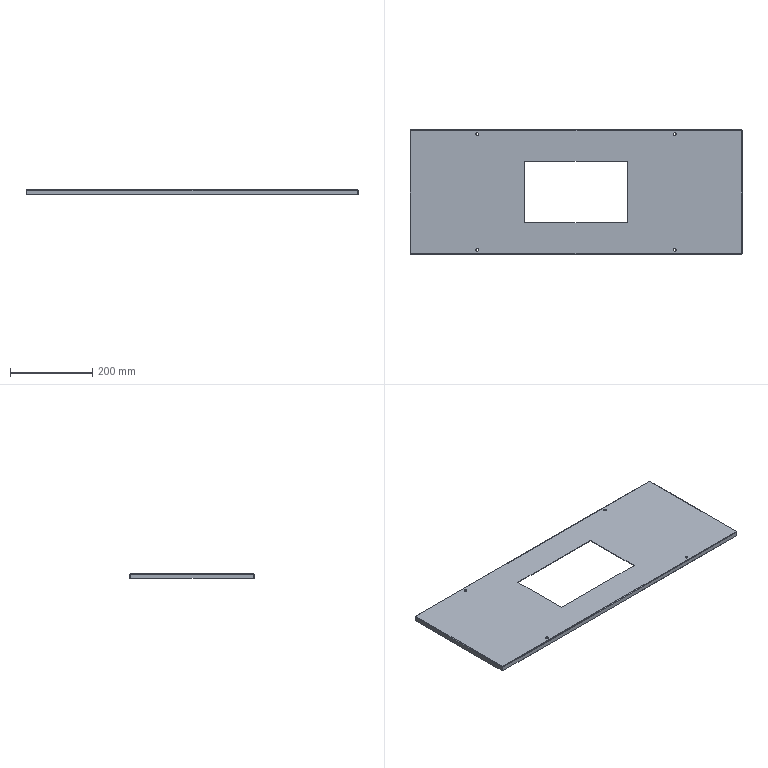Part | SolidWorks | features ICE 2, EdgeFlange 1, FlatPattern 1, SMBaseFlange 1, SheetMetal 1 | 1 solid | 50 faces | box 808 x 302 x 12 mm | volume 343087 mm3 | plane 26 | cylinder 16 | spline 8 | commonest cylinder face diameters 7 x8 0.2 x4 3.2 x4